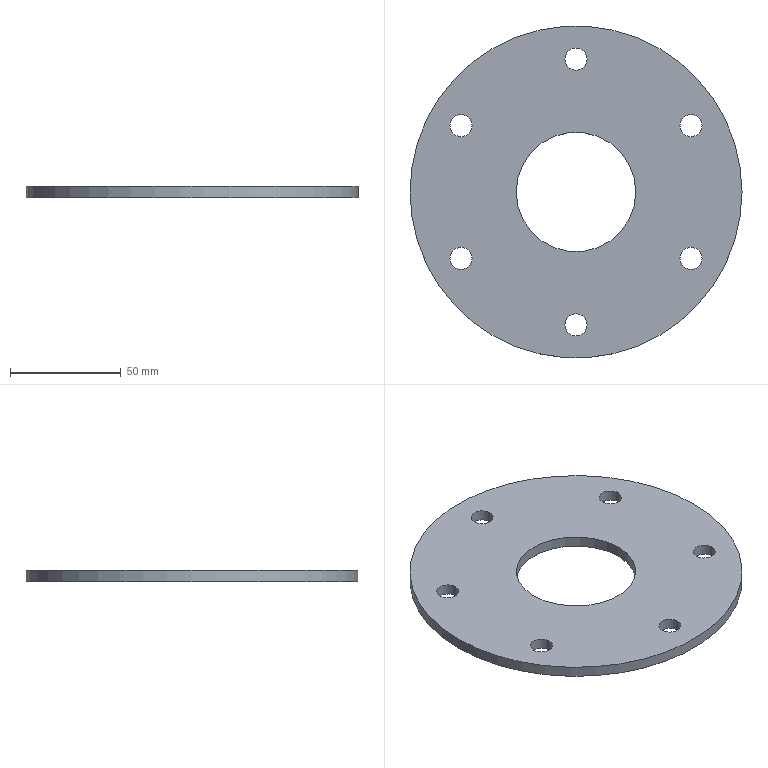Part | STEP file | JBJ-P-1012-02 | 1 solid | 10 faces | box 150 x 150 x 5 mm | volume 74550 mm3 | cylinder 8 | plane 2 | commonest cylinder face diameters 10 x6 54 x1 150 x1
STEP:
#1=CARTESIAN_POINT('',(-46.962,-30.,5.));
#2=VERTEX_POINT('',#1);
#3=CARTESIAN_POINT('',(-51.962,-30.,5.));
#4=DIRECTION('',(0.,0.,1.));
#5=DIRECTION('',(1.,0.,0.));
#6=AXIS2_PLACEMENT_3D('',#3,#4,#5);
#7=CIRCLE('',#6,5.);
#8=EDGE_CURVE('',#2,#2,#7,.T.);
#9=ORIENTED_EDGE('',*,*,#8,.F.);
#10=EDGE_LOOP('',(#9));
#11=FACE_BOUND('',#10,.T.);
#12=CARTESIAN_POINT('',(56.962,-30.,5.));
#13=VERTEX_POINT('',#12);
#14=CARTESIAN_POINT('',(51.962,-30.,5.));
#15=DIRECTION('',(0.,0.,1.));
#16=DIRECTION('',(1.,0.,0.));
#17=AXIS2_PLACEMENT_3D('',#14,#15,#16);
#18=CIRCLE('',#17,5.);
#19=EDGE_CURVE('',#13,#13,#18,.T.);
#20=ORIENTED_EDGE('',*,*,#19,.F.);
#21=EDGE_LOOP('',(#20));
#22=FACE_BOUND('',#21,.T.);
#23=CARTESIAN_POINT('',(5.,60.,5.));
#24=VERTEX_POINT('',#23);
#25=CARTESIAN_POINT('',(0.,60.,5.));
#26=DIRECTION('',(0.,0.,1.));
#27=DIRECTION('',(1.,0.,0.));
#28=AXIS2_PLACEMENT_3D('',#25,#26,#27);
#29=CIRCLE('',#28,5.);
#30=EDGE_CURVE('',#24,#24,#29,.T.);
#31=ORIENTED_EDGE('',*,*,#30,.F.);
#32=EDGE_LOOP('',(#31));
#33=FACE_BOUND('',#32,.T.);
#34=CARTESIAN_POINT('',(75.,0.,5.));
#35=VERTEX_POINT('',#34);
#36=CARTESIAN_POINT('',(0.,0.,5.));
#37=DIRECTION('',(0.,0.,1.));
#38=DIRECTION('',(1.,0.,0.));
#39=AXIS2_PLACEMENT_3D('',#36,#37,#38);
#40=CIRCLE('',#39,75.);
#41=EDGE_CURVE('',#35,#35,#40,.T.);
#42=ORIENTED_EDGE('',*,*,#41,.T.);
#43=EDGE_LOOP('',(#42));
#44=FACE_OUTER_BOUND('',#43,.T.);
#45=CARTESIAN_POINT('',(27.,0.,5.));
#46=VERTEX_POINT('',#45);
#47=CARTESIAN_POINT('',(0.,0.,5.));
#48=DIRECTION('',(0.,0.,1.));
#49=DIRECTION('',(1.,0.,0.));
#50=AXIS2_PLACEMENT_3D('',#47,#48,#49);
#51=CIRCLE('',#50,27.);
#52=EDGE_CURVE('',#46,#46,#51,.T.);
#53=ORIENTED_EDGE('',*,*,#52,.F.);
#54=EDGE_LOOP('',(#53));
#55=FACE_BOUND('',#54,.T.);
#56=CARTESIAN_POINT('',(56.962,30.,5.));
#57=VERTEX_POINT('',#56);
#58=CARTESIAN_POINT('',(51.962,30.,5.));
#59=DIRECTION('',(0.,0.,1.));
#60=DIRECTION('',(1.,0.,0.));
#61=AXIS2_PLACEMENT_3D('',#58,#59,#60);
#62=CIRCLE('',#61,5.);
#63=EDGE_CURVE('',#57,#57,#62,.T.);
#64=ORIENTED_EDGE('',*,*,#63,.F.);
#65=EDGE_LOOP('',(#64));
#66=FACE_BOUND('',#65,.T.);
#67=CARTESIAN_POINT('',(5.,-60.,5.));
#68=VERTEX_POINT('',#67);
#69=CARTESIAN_POINT('',(0.,-60.,5.));
#70=DIRECTION('',(0.,0.,1.));
#71=DIRECTION('',(1.,0.,0.));
#72=AXIS2_PLACEMENT_3D('',#69,#70,#71);
#73=CIRCLE('',#72,5.);
#74=EDGE_CURVE('',#68,#68,#73,.T.);
#75=ORIENTED_EDGE('',*,*,#74,.F.);
#76=EDGE_LOOP('',(#75));
#77=FACE_BOUND('',#76,.T.);
#78=CARTESIAN_POINT('',(-46.962,30.,5.));
#79=VERTEX_POINT('',#78);
#80=CARTESIAN_POINT('',(-51.962,30.,5.));
#81=DIRECTION('',(0.,0.,1.));
#82=DIRECTION('',(1.,0.,0.));
#83=AXIS2_PLACEMENT_3D('',#80,#81,#82);
#84=CIRCLE('',#83,5.);
#85=EDGE_CURVE('',#79,#79,#84,.T.);
#86=ORIENTED_EDGE('',*,*,#85,.F.);
#87=EDGE_LOOP('',(#86));
#88=FACE_BOUND('',#87,.T.);
#89=CARTESIAN_POINT('',(0.,0.,5.));
#90=DIRECTION('',(0.,0.,1.));
#91=DIRECTION('',(1.,0.,0.));
#92=AXIS2_PLACEMENT_3D('',#89,#90,#91);
#93=PLANE('',#92);
#94=ADVANCED_FACE('',(#11,#22,#33,#44,#55,#66,#77,#88),#93,.T.);
#95=CARTESIAN_POINT('',(75.,0.,0.));
#96=VERTEX_POINT('',#95);
#97=CARTESIAN_POINT('',(0.,0.,0.));
#98=DIRECTION('',(0.,0.,1.));
#99=DIRECTION('',(1.,0.,0.));
#100=AXIS2_PLACEMENT_3D('',#97,#98,#99);
#101=CIRCLE('',#100,75.);
#102=EDGE_CURVE('',#96,#96,#101,.T.);
#103=ORIENTED_EDGE('',*,*,#102,.F.);
#104=EDGE_LOOP('',(#103));
#105=FACE_OUTER_BOUND('',#104,.T.);
#106=CARTESIAN_POINT('',(27.,0.,0.));
#107=VERTEX_POINT('',#106);
#108=CARTESIAN_POINT('',(0.,0.,0.));
#109=DIRECTION('',(0.,0.,1.));
#110=DIRECTION('',(1.,0.,0.));
#111=AXIS2_PLACEMENT_3D('',#108,#109,#110);
#112=CIRCLE('',#111,27.);
#113=EDGE_CURVE('',#107,#107,#112,.T.);
#114=ORIENTED_EDGE('',*,*,#113,.T.);
#115=EDGE_LOOP('',(#114));
#116=FACE_BOUND('',#115,.T.);
#117=CARTESIAN_POINT('',(5.,60.,0.));
#118=VERTEX_POINT('',#117);
#119=CARTESIAN_POINT('',(0.,60.,0.));
#120=DIRECTION('',(0.,0.,1.));
#121=DIRECTION('',(1.,0.,0.));
#122=AXIS2_PLACEMENT_3D('',#119,#120,#121);
#123=CIRCLE('',#122,5.);
#124=EDGE_CURVE('',#118,#118,#123,.T.);
#125=ORIENTED_EDGE('',*,*,#124,.T.);
#126=EDGE_LOOP('',(#125));
#127=FACE_BOUND('',#126,.T.);
#128=CARTESIAN_POINT('',(56.962,30.,0.));
#129=VERTEX_POINT('',#128);
#130=CARTESIAN_POINT('',(51.962,30.,0.));
#131=DIRECTION('',(0.,0.,1.));
#132=DIRECTION('',(1.,0.,0.));
#133=AXIS2_PLACEMENT_3D('',#130,#131,#132);
#134=CIRCLE('',#133,5.);
#135=EDGE_CURVE('',#129,#129,#134,.T.);
#136=ORIENTED_EDGE('',*,*,#135,.T.);
#137=EDGE_LOOP('',(#136));
#138=FACE_BOUND('',#137,.T.);
#139=CARTESIAN_POINT('',(56.962,-30.,0.));
#140=VERTEX_POINT('',#139);
#141=CARTESIAN_POINT('',(51.962,-30.,0.));
#142=DIRECTION('',(0.,0.,1.));
#143=DIRECTION('',(1.,0.,0.));
#144=AXIS2_PLACEMENT_3D('',#141,#142,#143);
#145=CIRCLE('',#144,5.);
#146=EDGE_CURVE('',#140,#140,#145,.T.);
#147=ORIENTED_EDGE('',*,*,#146,.T.);
#148=EDGE_LOOP('',(#147));
#149=FACE_BOUND('',#148,.T.);
#150=CARTESIAN_POINT('',(5.,-60.,0.));
#151=VERTEX_POINT('',#150);
#152=CARTESIAN_POINT('',(0.,-60.,0.));
#153=DIRECTION('',(0.,0.,1.));
#154=DIRECTION('',(1.,0.,0.));
#155=AXIS2_PLACEMENT_3D('',#152,#153,#154);
#156=CIRCLE('',#155,5.);
#157=EDGE_CURVE('',#151,#151,#156,.T.);
#158=ORIENTED_EDGE('',*,*,#157,.T.);
#159=EDGE_LOOP('',(#158));
#160=FACE_BOUND('',#159,.T.);
#161=CARTESIAN_POINT('',(-46.962,-30.,0.));
#162=VERTEX_POINT('',#161);
#163=CARTESIAN_POINT('',(-51.962,-30.,0.));
#164=DIRECTION('',(0.,0.,1.));
#165=DIRECTION('',(1.,0.,0.));
#166=AXIS2_PLACEMENT_3D('',#163,#164,#165);
#167=CIRCLE('',#166,5.);
#168=EDGE_CURVE('',#162,#162,#167,.T.);
#169=ORIENTED_EDGE('',*,*,#168,.T.);
#170=EDGE_LOOP('',(#169));
#171=FACE_BOUND('',#170,.T.);
#172=CARTESIAN_POINT('',(-46.962,30.,0.));
#173=VERTEX_POINT('',#172);
#174=CARTESIAN_POINT('',(-51.962,30.,0.));
#175=DIRECTION('',(0.,0.,1.));
#176=DIRECTION('',(1.,0.,0.));
#177=AXIS2_PLACEMENT_3D('',#174,#175,#176);
#178=CIRCLE('',#177,5.);
#179=EDGE_CURVE('',#173,#173,#178,.T.);
#180=ORIENTED_EDGE('',*,*,#179,.T.);
#181=EDGE_LOOP('',(#180));
#182=FACE_BOUND('',#181,.T.);
#183=CARTESIAN_POINT('',(0.,0.,0.));
#184=DIRECTION('',(0.,0.,1.));
#185=DIRECTION('',(1.,0.,0.));
#186=AXIS2_PLACEMENT_3D('',#183,#184,#185);
#187=PLANE('',#186);
#188=ADVANCED_FACE('',(#105,#116,#127,#138,#149,#160,#171,#182),#187,.F.);
#189=ORIENTED_EDGE('',*,*,#41,.F.);
#190=EDGE_LOOP('',(#189));
#191=FACE_OUTER_BOUND('',#190,.T.);
#192=ORIENTED_EDGE('',*,*,#102,.T.);
#193=EDGE_LOOP('',(#192));
#194=FACE_OUTER_BOUND('',#193,.T.);
#195=CARTESIAN_POINT('',(0.,0.,5.));
#196=DIRECTION('',(0.,0.,-1.));
#197=DIRECTION('',(-1.,0.,0.));
#198=AXIS2_PLACEMENT_3D('',#195,#196,#197);
#199=CYLINDRICAL_SURFACE('',#198,75.);
#200=ADVANCED_FACE('',(#191,#194),#199,.T.);
#201=ORIENTED_EDGE('',*,*,#52,.T.);
#202=EDGE_LOOP('',(#201));
#203=FACE_OUTER_BOUND('',#202,.T.);
#204=ORIENTED_EDGE('',*,*,#113,.F.);
#205=EDGE_LOOP('',(#204));
#206=FACE_OUTER_BOUND('',#205,.T.);
#207=CARTESIAN_POINT('',(0.,0.,5.));
#208=DIRECTION('',(0.,0.,-1.));
#209=DIRECTION('',(-1.,0.,0.));
#210=AXIS2_PLACEMENT_3D('',#207,#208,#209);
#211=CYLINDRICAL_SURFACE('',#210,27.);
#212=ADVANCED_FACE('',(#203,#206),#211,.F.);
#213=ORIENTED_EDGE('',*,*,#30,.T.);
#214=EDGE_LOOP('',(#213));
#215=FACE_OUTER_BOUND('',#214,.T.);
#216=ORIENTED_EDGE('',*,*,#124,.F.);
#217=EDGE_LOOP('',(#216));
#218=FACE_OUTER_BOUND('',#217,.T.);
#219=CARTESIAN_POINT('',(0.,60.,5.));
#220=DIRECTION('',(0.,0.,-1.));
#221=DIRECTION('',(-1.,0.,0.));
#222=AXIS2_PLACEMENT_3D('',#219,#220,#221);
#223=CYLINDRICAL_SURFACE('',#222,5.);
#224=ADVANCED_FACE('',(#215,#218),#223,.F.);
#225=ORIENTED_EDGE('',*,*,#63,.T.);
#226=EDGE_LOOP('',(#225));
#227=FACE_OUTER_BOUND('',#226,.T.);
#228=ORIENTED_EDGE('',*,*,#135,.F.);
#229=EDGE_LOOP('',(#228));
#230=FACE_OUTER_BOUND('',#229,.T.);
#231=CARTESIAN_POINT('',(51.962,30.,5.));
#232=DIRECTION('',(0.,0.,-1.));
#233=DIRECTION('',(-1.,0.,0.));
#234=AXIS2_PLACEMENT_3D('',#231,#232,#233);
#235=CYLINDRICAL_SURFACE('',#234,5.);
#236=ADVANCED_FACE('',(#227,#230),#235,.F.);
#237=ORIENTED_EDGE('',*,*,#19,.T.);
#238=EDGE_LOOP('',(#237));
#239=FACE_OUTER_BOUND('',#238,.T.);
#240=ORIENTED_EDGE('',*,*,#146,.F.);
#241=EDGE_LOOP('',(#240));
#242=FACE_OUTER_BOUND('',#241,.T.);
#243=CARTESIAN_POINT('',(51.962,-30.,5.));
#244=DIRECTION('',(0.,0.,-1.));
#245=DIRECTION('',(-1.,0.,0.));
#246=AXIS2_PLACEMENT_3D('',#243,#244,#245);
#247=CYLINDRICAL_SURFACE('',#246,5.);
#248=ADVANCED_FACE('',(#239,#242),#247,.F.);
#249=ORIENTED_EDGE('',*,*,#74,.T.);
#250=EDGE_LOOP('',(#249));
#251=FACE_OUTER_BOUND('',#250,.T.);
#252=ORIENTED_EDGE('',*,*,#157,.F.);
#253=EDGE_LOOP('',(#252));
#254=FACE_OUTER_BOUND('',#253,.T.);
#255=CARTESIAN_POINT('',(0.,-60.,5.));
#256=DIRECTION('',(0.,0.,-1.));
#257=DIRECTION('',(-1.,0.,0.));
#258=AXIS2_PLACEMENT_3D('',#255,#256,#257);
#259=CYLINDRICAL_SURFACE('',#258,5.);
#260=ADVANCED_FACE('',(#251,#254),#259,.F.);
#261=ORIENTED_EDGE('',*,*,#8,.T.);
#262=EDGE_LOOP('',(#261));
#263=FACE_OUTER_BOUND('',#262,.T.);
#264=ORIENTED_EDGE('',*,*,#168,.F.);
#265=EDGE_LOOP('',(#264));
#266=FACE_OUTER_BOUND('',#265,.T.);
#267=CARTESIAN_POINT('',(-51.962,-30.,5.));
#268=DIRECTION('',(0.,0.,-1.));
#269=DIRECTION('',(-1.,0.,0.));
#270=AXIS2_PLACEMENT_3D('',#267,#268,#269);
#271=CYLINDRICAL_SURFACE('',#270,5.);
#272=ADVANCED_FACE('',(#263,#266),#271,.F.);
#273=ORIENTED_EDGE('',*,*,#85,.T.);
#274=EDGE_LOOP('',(#273));
#275=FACE_OUTER_BOUND('',#274,.T.);
#276=ORIENTED_EDGE('',*,*,#179,.F.);
#277=EDGE_LOOP('',(#276));
#278=FACE_OUTER_BOUND('',#277,.T.);
#279=CARTESIAN_POINT('',(-51.962,30.,5.));
#280=DIRECTION('',(0.,0.,-1.));
#281=DIRECTION('',(-1.,0.,0.));
#282=AXIS2_PLACEMENT_3D('',#279,#280,#281);
#283=CYLINDRICAL_SURFACE('',#282,5.);
#284=ADVANCED_FACE('',(#275,#278),#283,.F.);
#285=CLOSED_SHELL('',(#94,#188,#200,#212,#224,#236,#248,#260,#272,#284));
#286=MANIFOLD_SOLID_BREP('',#285);
#287=CARTESIAN_POINT('',(0.,0.,0.));
#288=DIRECTION('',(0.,0.,1.));
#289=DIRECTION('',(1.,0.,0.));
#290=AXIS2_PLACEMENT_3D('',#287,#288,#289);
#291=(LENGTH_UNIT()NAMED_UNIT(*)SI_UNIT(.MILLI.,.METRE.));
#292=UNCERTAINTY_MEASURE_WITH_UNIT(LENGTH_MEASURE(0.00001),#291,'','');
#293=(NAMED_UNIT(*)PLANE_ANGLE_UNIT()SI_UNIT($,.RADIAN.));
#294=(NAMED_UNIT(*)SI_UNIT($,.STERADIAN.)SOLID_ANGLE_UNIT());
#295=(GEOMETRIC_REPRESENTATION_CONTEXT(3)GLOBAL_UNCERTAINTY_ASSIGNED_CONTEXT((#292))GLOBAL_UNIT_ASSIGNED_CONTEXT((#291,#293,#294))REPRESENTATION_CONTEXT('',''));
#296=ADVANCED_BREP_SHAPE_REPRESENTATION('',(#286,#290),#295);